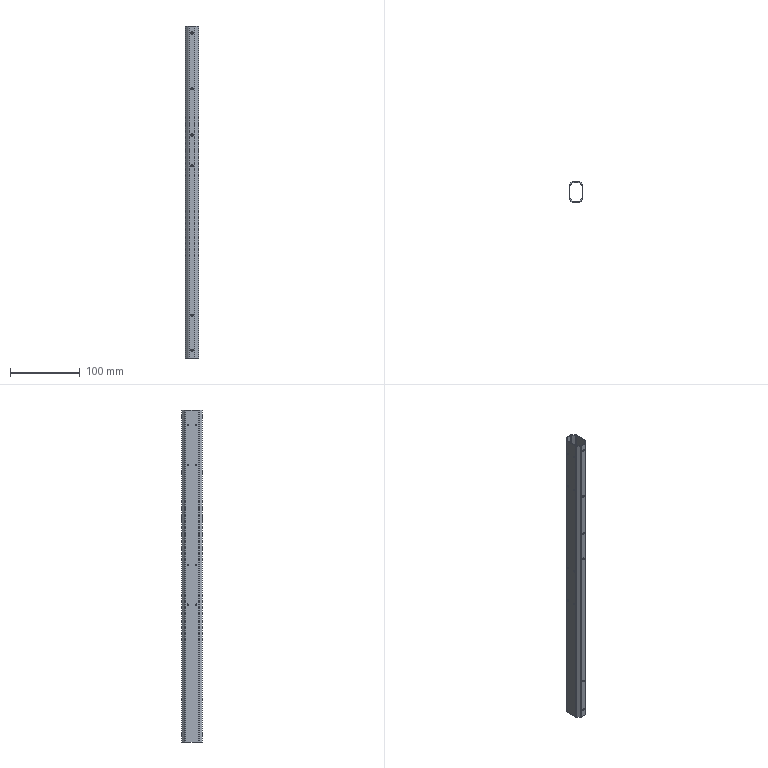Part | SolidWorks | features ICE 3, Fillet 2, Extrusion 1 | 1 solid | 122 faces | box 20 x 30 x 475 mm | volume 40009 mm3 | cylinder 96 | plane 26 | commonest cylinder face diameters 3.1 x24 7 x24 2 x16 2.1 x16 4 x16